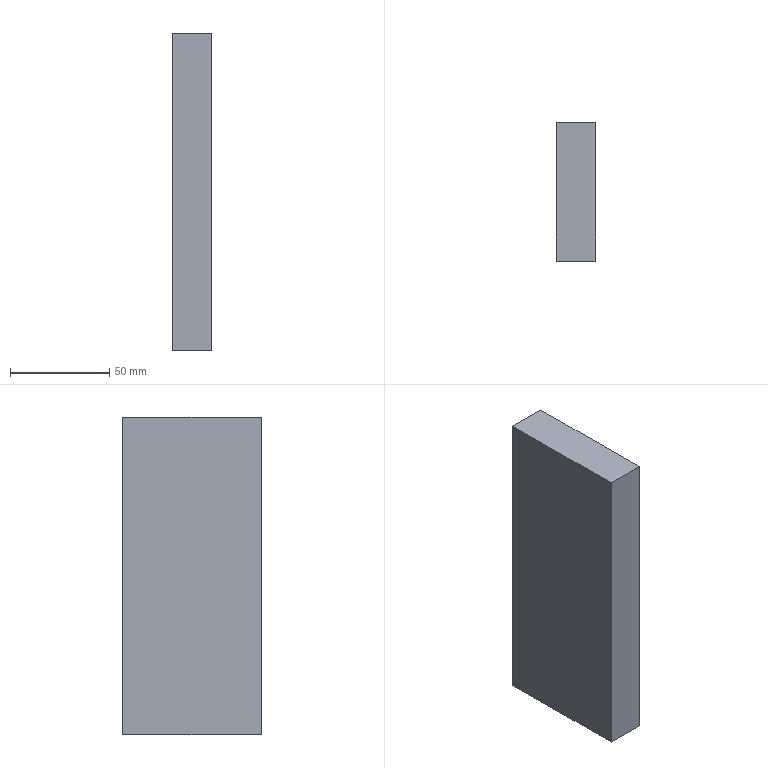Part | STEP file | Part 1 | 1 solid | 6 faces | box 20 x 70 x 160 mm | volume 224000 mm3 | plane 6
STEP:
#1=CARTESIAN_POINT('',(0.,0.,0.));
#2=DIRECTION('',(0.,0.,1.));
#3=DIRECTION('',(1.,0.,0.));
#4=AXIS2_PLACEMENT_3D('',#1,#2,#3);
#5=CARTESIAN_POINT('',(40.,60.,-80.));
#6=VERTEX_POINT('',#5);
#7=CARTESIAN_POINT('',(40.,60.,80.));
#8=VERTEX_POINT('',#7);
#9=CARTESIAN_POINT('',(40.,60.,-80.));
#10=DIRECTION('',(0.,0.,1.));
#11=VECTOR('',#10,1.);
#12=LINE('',#9,#11);
#13=CARTESIAN_POINT('',(20.,60.,-80.));
#14=DIRECTION('',(0.,1.,0.));
#15=DIRECTION('',(0.,0.,1.));
#16=AXIS2_PLACEMENT_3D('',#13,#14,#15);
#17=PLANE('',#16);
#18=CARTESIAN_POINT('',(0.,20.));
#19=DIRECTION('',(1.,0.));
#20=VECTOR('',#19,1.);
#21=LINE('',#18,#20);
#22=(GEOMETRIC_REPRESENTATION_CONTEXT(2)PARAMETRIC_REPRESENTATION_CONTEXT()REPRESENTATION_CONTEXT('',''));
#23=DEFINITIONAL_REPRESENTATION('',(#21),#22);
#24=PCURVE('',#17,#23);
#25=CARTESIAN_POINT('',(40.,0.,0.));
#26=DIRECTION('',(1.,0.,0.));
#27=DIRECTION('',(0.,0.,-1.));
#28=AXIS2_PLACEMENT_3D('',#25,#26,#27);
#29=PLANE('',#28);
#30=CARTESIAN_POINT('',(80.,60.));
#31=DIRECTION('',(-1.,0.));
#32=VECTOR('',#31,1.);
#33=LINE('',#30,#32);
#34=(GEOMETRIC_REPRESENTATION_CONTEXT(2)PARAMETRIC_REPRESENTATION_CONTEXT()REPRESENTATION_CONTEXT('',''));
#35=DEFINITIONAL_REPRESENTATION('',(#33),#34);
#36=PCURVE('',#29,#35);
#37=SURFACE_CURVE('',#12,(#24,#36),.PCURVE_S1.);
#38=EDGE_CURVE('',#6,#8,#37,.T.);
#39=ORIENTED_EDGE('',*,*,#38,.F.);
#40=CARTESIAN_POINT('',(20.,60.,-80.));
#41=VERTEX_POINT('',#40);
#42=CARTESIAN_POINT('',(20.,60.,-80.));
#43=DIRECTION('',(1.,0.,0.));
#44=VECTOR('',#43,1.);
#45=LINE('',#42,#44);
#46=CARTESIAN_POINT('',(0.,0.));
#47=DIRECTION('',(0.,1.));
#48=VECTOR('',#47,1.);
#49=LINE('',#46,#48);
#50=(GEOMETRIC_REPRESENTATION_CONTEXT(2)PARAMETRIC_REPRESENTATION_CONTEXT()REPRESENTATION_CONTEXT('',''));
#51=DEFINITIONAL_REPRESENTATION('',(#49),#50);
#52=PCURVE('',#17,#51);
#53=CARTESIAN_POINT('',(20.,-10.,-80.));
#54=DIRECTION('',(0.,0.,-1.));
#55=DIRECTION('',(-1.,0.,0.));
#56=AXIS2_PLACEMENT_3D('',#53,#54,#55);
#57=PLANE('',#56);
#58=CARTESIAN_POINT('',(0.,70.));
#59=DIRECTION('',(-1.,0.));
#60=VECTOR('',#59,1.);
#61=LINE('',#58,#60);
#62=(GEOMETRIC_REPRESENTATION_CONTEXT(2)PARAMETRIC_REPRESENTATION_CONTEXT()REPRESENTATION_CONTEXT('',''));
#63=DEFINITIONAL_REPRESENTATION('',(#61),#62);
#64=PCURVE('',#57,#63);
#65=SURFACE_CURVE('',#45,(#52,#64),.PCURVE_S1.);
#66=EDGE_CURVE('',#41,#6,#65,.T.);
#67=ORIENTED_EDGE('',*,*,#66,.F.);
#68=CARTESIAN_POINT('',(20.,60.,80.));
#69=VERTEX_POINT('',#68);
#70=CARTESIAN_POINT('',(20.,60.,-80.));
#71=DIRECTION('',(0.,0.,1.));
#72=VECTOR('',#71,1.);
#73=LINE('',#70,#72);
#74=CARTESIAN_POINT('',(0.,0.));
#75=DIRECTION('',(1.,0.));
#76=VECTOR('',#75,1.);
#77=LINE('',#74,#76);
#78=(GEOMETRIC_REPRESENTATION_CONTEXT(2)PARAMETRIC_REPRESENTATION_CONTEXT()REPRESENTATION_CONTEXT('',''));
#79=DEFINITIONAL_REPRESENTATION('',(#77),#78);
#80=PCURVE('',#17,#79);
#81=CARTESIAN_POINT('',(20.,0.,0.));
#82=DIRECTION('',(1.,0.,0.));
#83=DIRECTION('',(0.,0.,-1.));
#84=AXIS2_PLACEMENT_3D('',#81,#82,#83);
#85=PLANE('',#84);
#86=CARTESIAN_POINT('',(80.,60.));
#87=DIRECTION('',(-1.,0.));
#88=VECTOR('',#87,1.);
#89=LINE('',#86,#88);
#90=(GEOMETRIC_REPRESENTATION_CONTEXT(2)PARAMETRIC_REPRESENTATION_CONTEXT()REPRESENTATION_CONTEXT('',''));
#91=DEFINITIONAL_REPRESENTATION('',(#89),#90);
#92=PCURVE('',#85,#91);
#93=SURFACE_CURVE('',#73,(#80,#92),.PCURVE_S1.);
#94=EDGE_CURVE('',#41,#69,#93,.T.);
#95=ORIENTED_EDGE('',*,*,#94,.T.);
#96=CARTESIAN_POINT('',(20.,60.,80.));
#97=DIRECTION('',(1.,0.,0.));
#98=VECTOR('',#97,1.);
#99=LINE('',#96,#98);
#100=CARTESIAN_POINT('',(160.,0.));
#101=DIRECTION('',(0.,1.));
#102=VECTOR('',#101,1.);
#103=LINE('',#100,#102);
#104=(GEOMETRIC_REPRESENTATION_CONTEXT(2)PARAMETRIC_REPRESENTATION_CONTEXT()REPRESENTATION_CONTEXT('',''));
#105=DEFINITIONAL_REPRESENTATION('',(#103),#104);
#106=PCURVE('',#17,#105);
#107=CARTESIAN_POINT('',(20.,60.,80.));
#108=DIRECTION('',(0.,0.,1.));
#109=DIRECTION('',(1.,0.,0.));
#110=AXIS2_PLACEMENT_3D('',#107,#108,#109);
#111=PLANE('',#110);
#112=CARTESIAN_POINT('',(0.,0.));
#113=DIRECTION('',(1.,0.));
#114=VECTOR('',#113,1.);
#115=LINE('',#112,#114);
#116=(GEOMETRIC_REPRESENTATION_CONTEXT(2)PARAMETRIC_REPRESENTATION_CONTEXT()REPRESENTATION_CONTEXT('',''));
#117=DEFINITIONAL_REPRESENTATION('',(#115),#116);
#118=PCURVE('',#111,#117);
#119=SURFACE_CURVE('',#99,(#106,#118),.PCURVE_S1.);
#120=EDGE_CURVE('',#69,#8,#119,.T.);
#121=ORIENTED_EDGE('',*,*,#120,.T.);
#122=EDGE_LOOP('',(#39,#67,#95,#121));
#123=FACE_BOUND('',#122,.T.);
#124=ADVANCED_FACE('',(#123),#17,.T.);
#125=CARTESIAN_POINT('',(40.,-10.,-80.));
#126=VERTEX_POINT('',#125);
#127=CARTESIAN_POINT('',(40.,-10.,-80.));
#128=DIRECTION('',(0.,1.,0.));
#129=VECTOR('',#128,1.);
#130=LINE('',#127,#129);
#131=CARTESIAN_POINT('',(-20.,0.));
#132=DIRECTION('',(0.,1.));
#133=VECTOR('',#132,1.);
#134=LINE('',#131,#133);
#135=(GEOMETRIC_REPRESENTATION_CONTEXT(2)PARAMETRIC_REPRESENTATION_CONTEXT()REPRESENTATION_CONTEXT('',''));
#136=DEFINITIONAL_REPRESENTATION('',(#134),#135);
#137=PCURVE('',#57,#136);
#138=CARTESIAN_POINT('',(80.,-10.));
#139=DIRECTION('',(0.,1.));
#140=VECTOR('',#139,1.);
#141=LINE('',#138,#140);
#142=(GEOMETRIC_REPRESENTATION_CONTEXT(2)PARAMETRIC_REPRESENTATION_CONTEXT()REPRESENTATION_CONTEXT('',''));
#143=DEFINITIONAL_REPRESENTATION('',(#141),#142);
#144=PCURVE('',#29,#143);
#145=SURFACE_CURVE('',#130,(#137,#144),.PCURVE_S1.);
#146=EDGE_CURVE('',#126,#6,#145,.T.);
#147=ORIENTED_EDGE('',*,*,#146,.F.);
#148=CARTESIAN_POINT('',(20.,-10.,-80.));
#149=VERTEX_POINT('',#148);
#150=CARTESIAN_POINT('',(20.,-10.,-80.));
#151=DIRECTION('',(1.,0.,0.));
#152=VECTOR('',#151,1.);
#153=LINE('',#150,#152);
#154=CARTESIAN_POINT('',(0.,0.));
#155=DIRECTION('',(-1.,0.));
#156=VECTOR('',#155,1.);
#157=LINE('',#154,#156);
#158=(GEOMETRIC_REPRESENTATION_CONTEXT(2)PARAMETRIC_REPRESENTATION_CONTEXT()REPRESENTATION_CONTEXT('',''));
#159=DEFINITIONAL_REPRESENTATION('',(#157),#158);
#160=PCURVE('',#57,#159);
#161=CARTESIAN_POINT('',(20.,-10.,80.));
#162=DIRECTION('',(0.,-1.,0.));
#163=DIRECTION('',(0.,0.,-1.));
#164=AXIS2_PLACEMENT_3D('',#161,#162,#163);
#165=PLANE('',#164);
#166=CARTESIAN_POINT('',(160.,0.));
#167=DIRECTION('',(0.,1.));
#168=VECTOR('',#167,1.);
#169=LINE('',#166,#168);
#170=(GEOMETRIC_REPRESENTATION_CONTEXT(2)PARAMETRIC_REPRESENTATION_CONTEXT()REPRESENTATION_CONTEXT('',''));
#171=DEFINITIONAL_REPRESENTATION('',(#169),#170);
#172=PCURVE('',#165,#171);
#173=SURFACE_CURVE('',#153,(#160,#172),.PCURVE_S1.);
#174=EDGE_CURVE('',#149,#126,#173,.T.);
#175=ORIENTED_EDGE('',*,*,#174,.F.);
#176=CARTESIAN_POINT('',(20.,-10.,-80.));
#177=DIRECTION('',(0.,1.,0.));
#178=VECTOR('',#177,1.);
#179=LINE('',#176,#178);
#180=CARTESIAN_POINT('',(0.,0.));
#181=DIRECTION('',(0.,1.));
#182=VECTOR('',#181,1.);
#183=LINE('',#180,#182);
#184=(GEOMETRIC_REPRESENTATION_CONTEXT(2)PARAMETRIC_REPRESENTATION_CONTEXT()REPRESENTATION_CONTEXT('',''));
#185=DEFINITIONAL_REPRESENTATION('',(#183),#184);
#186=PCURVE('',#57,#185);
#187=CARTESIAN_POINT('',(80.,-10.));
#188=DIRECTION('',(0.,1.));
#189=VECTOR('',#188,1.);
#190=LINE('',#187,#189);
#191=(GEOMETRIC_REPRESENTATION_CONTEXT(2)PARAMETRIC_REPRESENTATION_CONTEXT()REPRESENTATION_CONTEXT('',''));
#192=DEFINITIONAL_REPRESENTATION('',(#190),#191);
#193=PCURVE('',#85,#192);
#194=SURFACE_CURVE('',#179,(#186,#193),.PCURVE_S1.);
#195=EDGE_CURVE('',#149,#41,#194,.T.);
#196=ORIENTED_EDGE('',*,*,#195,.T.);
#197=ORIENTED_EDGE('',*,*,#66,.T.);
#198=EDGE_LOOP('',(#147,#175,#196,#197));
#199=FACE_BOUND('',#198,.T.);
#200=ADVANCED_FACE('',(#199),#57,.T.);
#201=CARTESIAN_POINT('',(40.,-10.,80.));
#202=VERTEX_POINT('',#201);
#203=CARTESIAN_POINT('',(40.,-10.,80.));
#204=DIRECTION('',(0.,0.,-1.));
#205=VECTOR('',#204,1.);
#206=LINE('',#203,#205);
#207=CARTESIAN_POINT('',(0.,20.));
#208=DIRECTION('',(1.,0.));
#209=VECTOR('',#208,1.);
#210=LINE('',#207,#209);
#211=(GEOMETRIC_REPRESENTATION_CONTEXT(2)PARAMETRIC_REPRESENTATION_CONTEXT()REPRESENTATION_CONTEXT('',''));
#212=DEFINITIONAL_REPRESENTATION('',(#210),#211);
#213=PCURVE('',#165,#212);
#214=CARTESIAN_POINT('',(-80.,-10.));
#215=DIRECTION('',(1.,0.));
#216=VECTOR('',#215,1.);
#217=LINE('',#214,#216);
#218=(GEOMETRIC_REPRESENTATION_CONTEXT(2)PARAMETRIC_REPRESENTATION_CONTEXT()REPRESENTATION_CONTEXT('',''));
#219=DEFINITIONAL_REPRESENTATION('',(#217),#218);
#220=PCURVE('',#29,#219);
#221=SURFACE_CURVE('',#206,(#213,#220),.PCURVE_S1.);
#222=EDGE_CURVE('',#202,#126,#221,.T.);
#223=ORIENTED_EDGE('',*,*,#222,.F.);
#224=CARTESIAN_POINT('',(20.,-10.,80.));
#225=VERTEX_POINT('',#224);
#226=CARTESIAN_POINT('',(20.,-10.,80.));
#227=DIRECTION('',(1.,0.,0.));
#228=VECTOR('',#227,1.);
#229=LINE('',#226,#228);
#230=CARTESIAN_POINT('',(0.,0.));
#231=DIRECTION('',(0.,1.));
#232=VECTOR('',#231,1.);
#233=LINE('',#230,#232);
#234=(GEOMETRIC_REPRESENTATION_CONTEXT(2)PARAMETRIC_REPRESENTATION_CONTEXT()REPRESENTATION_CONTEXT('',''));
#235=DEFINITIONAL_REPRESENTATION('',(#233),#234);
#236=PCURVE('',#165,#235);
#237=CARTESIAN_POINT('',(0.,-70.));
#238=DIRECTION('',(1.,0.));
#239=VECTOR('',#238,1.);
#240=LINE('',#237,#239);
#241=(GEOMETRIC_REPRESENTATION_CONTEXT(2)PARAMETRIC_REPRESENTATION_CONTEXT()REPRESENTATION_CONTEXT('',''));
#242=DEFINITIONAL_REPRESENTATION('',(#240),#241);
#243=PCURVE('',#111,#242);
#244=SURFACE_CURVE('',#229,(#236,#243),.PCURVE_S1.);
#245=EDGE_CURVE('',#225,#202,#244,.T.);
#246=ORIENTED_EDGE('',*,*,#245,.F.);
#247=CARTESIAN_POINT('',(20.,-10.,80.));
#248=DIRECTION('',(0.,0.,-1.));
#249=VECTOR('',#248,1.);
#250=LINE('',#247,#249);
#251=CARTESIAN_POINT('',(0.,0.));
#252=DIRECTION('',(1.,0.));
#253=VECTOR('',#252,1.);
#254=LINE('',#251,#253);
#255=(GEOMETRIC_REPRESENTATION_CONTEXT(2)PARAMETRIC_REPRESENTATION_CONTEXT()REPRESENTATION_CONTEXT('',''));
#256=DEFINITIONAL_REPRESENTATION('',(#254),#255);
#257=PCURVE('',#165,#256);
#258=CARTESIAN_POINT('',(-80.,-10.));
#259=DIRECTION('',(1.,0.));
#260=VECTOR('',#259,1.);
#261=LINE('',#258,#260);
#262=(GEOMETRIC_REPRESENTATION_CONTEXT(2)PARAMETRIC_REPRESENTATION_CONTEXT()REPRESENTATION_CONTEXT('',''));
#263=DEFINITIONAL_REPRESENTATION('',(#261),#262);
#264=PCURVE('',#85,#263);
#265=SURFACE_CURVE('',#250,(#257,#264),.PCURVE_S1.);
#266=EDGE_CURVE('',#225,#149,#265,.T.);
#267=ORIENTED_EDGE('',*,*,#266,.T.);
#268=ORIENTED_EDGE('',*,*,#174,.T.);
#269=EDGE_LOOP('',(#223,#246,#267,#268));
#270=FACE_BOUND('',#269,.T.);
#271=ADVANCED_FACE('',(#270),#165,.T.);
#272=CARTESIAN_POINT('',(40.,60.,80.));
#273=DIRECTION('',(0.,-1.,0.));
#274=VECTOR('',#273,1.);
#275=LINE('',#272,#274);
#276=CARTESIAN_POINT('',(20.,0.));
#277=DIRECTION('',(0.,-1.));
#278=VECTOR('',#277,1.);
#279=LINE('',#276,#278);
#280=(GEOMETRIC_REPRESENTATION_CONTEXT(2)PARAMETRIC_REPRESENTATION_CONTEXT()REPRESENTATION_CONTEXT('',''));
#281=DEFINITIONAL_REPRESENTATION('',(#279),#280);
#282=PCURVE('',#111,#281);
#283=CARTESIAN_POINT('',(-80.,60.));
#284=DIRECTION('',(0.,-1.));
#285=VECTOR('',#284,1.);
#286=LINE('',#283,#285);
#287=(GEOMETRIC_REPRESENTATION_CONTEXT(2)PARAMETRIC_REPRESENTATION_CONTEXT()REPRESENTATION_CONTEXT('',''));
#288=DEFINITIONAL_REPRESENTATION('',(#286),#287);
#289=PCURVE('',#29,#288);
#290=SURFACE_CURVE('',#275,(#282,#289),.PCURVE_S1.);
#291=EDGE_CURVE('',#8,#202,#290,.T.);
#292=ORIENTED_EDGE('',*,*,#291,.F.);
#293=ORIENTED_EDGE('',*,*,#120,.F.);
#294=CARTESIAN_POINT('',(20.,60.,80.));
#295=DIRECTION('',(0.,-1.,0.));
#296=VECTOR('',#295,1.);
#297=LINE('',#294,#296);
#298=CARTESIAN_POINT('',(0.,0.));
#299=DIRECTION('',(0.,-1.));
#300=VECTOR('',#299,1.);
#301=LINE('',#298,#300);
#302=(GEOMETRIC_REPRESENTATION_CONTEXT(2)PARAMETRIC_REPRESENTATION_CONTEXT()REPRESENTATION_CONTEXT('',''));
#303=DEFINITIONAL_REPRESENTATION('',(#301),#302);
#304=PCURVE('',#111,#303);
#305=CARTESIAN_POINT('',(-80.,60.));
#306=DIRECTION('',(0.,-1.));
#307=VECTOR('',#306,1.);
#308=LINE('',#305,#307);
#309=(GEOMETRIC_REPRESENTATION_CONTEXT(2)PARAMETRIC_REPRESENTATION_CONTEXT()REPRESENTATION_CONTEXT('',''));
#310=DEFINITIONAL_REPRESENTATION('',(#308),#309);
#311=PCURVE('',#85,#310);
#312=SURFACE_CURVE('',#297,(#304,#311),.PCURVE_S1.);
#313=EDGE_CURVE('',#69,#225,#312,.T.);
#314=ORIENTED_EDGE('',*,*,#313,.T.);
#315=ORIENTED_EDGE('',*,*,#245,.T.);
#316=EDGE_LOOP('',(#292,#293,#314,#315));
#317=FACE_BOUND('',#316,.T.);
#318=ADVANCED_FACE('',(#317),#111,.T.);
#319=ORIENTED_EDGE('',*,*,#94,.F.);
#320=ORIENTED_EDGE('',*,*,#195,.F.);
#321=ORIENTED_EDGE('',*,*,#266,.F.);
#322=ORIENTED_EDGE('',*,*,#313,.F.);
#323=EDGE_LOOP('',(#319,#320,#321,#322));
#324=FACE_BOUND('',#323,.T.);
#325=ADVANCED_FACE('',(#324),#85,.F.);
#326=ORIENTED_EDGE('',*,*,#38,.T.);
#327=ORIENTED_EDGE('',*,*,#291,.T.);
#328=ORIENTED_EDGE('',*,*,#222,.T.);
#329=ORIENTED_EDGE('',*,*,#146,.T.);
#330=EDGE_LOOP('',(#326,#327,#328,#329));
#331=FACE_BOUND('',#330,.T.);
#332=ADVANCED_FACE('',(#331),#29,.T.);
#333=CLOSED_SHELL('',(#124,#200,#271,#318,#325,#332));
#334=MANIFOLD_SOLID_BREP('',#333);
#335=(LENGTH_UNIT()NAMED_UNIT(*)SI_UNIT(.MILLI.,.METRE.));
#336=UNCERTAINTY_MEASURE_WITH_UNIT(LENGTH_MEASURE(0.0000001),#335,'','');
#337=(NAMED_UNIT(*)PLANE_ANGLE_UNIT()SI_UNIT($,.RADIAN.));
#338=(NAMED_UNIT(*)SI_UNIT($,.STERADIAN.)SOLID_ANGLE_UNIT());
#339=(GEOMETRIC_REPRESENTATION_CONTEXT(3)GLOBAL_UNCERTAINTY_ASSIGNED_CONTEXT((#336))GLOBAL_UNIT_ASSIGNED_CONTEXT((#335,#337,#338))REPRESENTATION_CONTEXT('',''));
#340=ADVANCED_BREP_SHAPE_REPRESENTATION('',(#4,#334),#339);